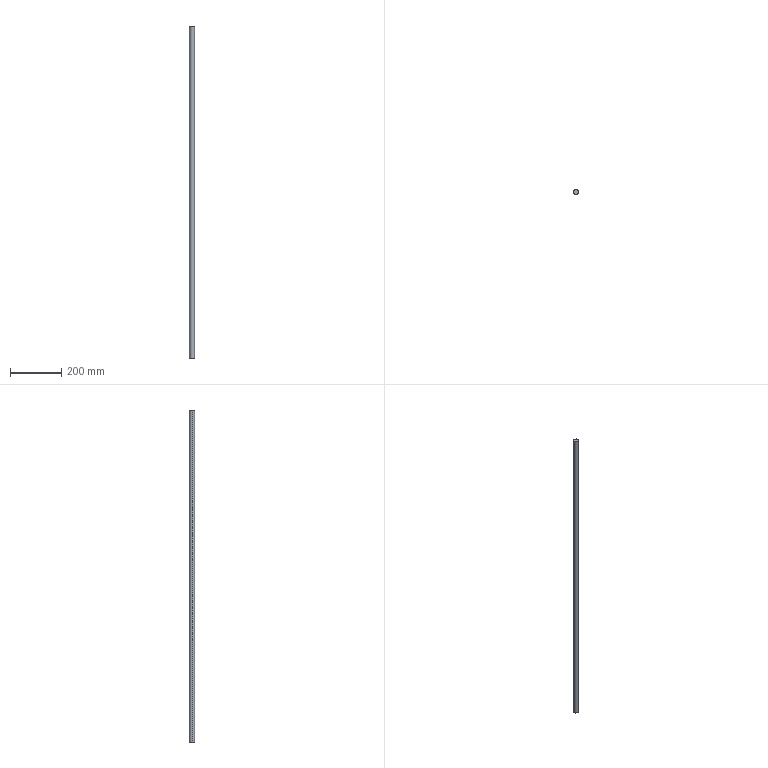Part | SolidWorks | features Extrusion 1 | 1 solid | 4 faces | box 20 x 20 x 1300 mm | volume 408407 mm3 | cylinder 2 | plane 2 | commonest cylinder face diameters 20 x2
STEP:
#1=CARTESIAN_POINT('',(10.,0.,650.));
#2=VERTEX_POINT('',#1);
#3=CARTESIAN_POINT('',(-10.,0.,650.));
#4=VERTEX_POINT('',#3);
#5=CARTESIAN_POINT('',(0.,0.,650.));
#6=DIRECTION('',(0.,0.,1.));
#7=DIRECTION('',(1.,0.,0.));
#8=AXIS2_PLACEMENT_3D('',#5,#6,#7);
#9=CIRCLE('',#8,10.);
#10=EDGE_CURVE('',#2,#4,#9,.T.);
#11=ORIENTED_EDGE('',*,*,#10,.F.);
#12=CARTESIAN_POINT('',(10.,0.,-650.));
#13=VERTEX_POINT('',#12);
#14=CARTESIAN_POINT('',(10.,0.,650.));
#15=DIRECTION('',(0.,0.,-1.));
#16=VECTOR('',#15,1000.);
#17=LINE('',#14,#16);
#18=EDGE_CURVE('',#2,#13,#17,.T.);
#19=ORIENTED_EDGE('',*,*,#18,.T.);
#20=CARTESIAN_POINT('',(-10.,0.,-650.));
#21=VERTEX_POINT('',#20);
#22=CARTESIAN_POINT('',(0.,0.,-650.));
#23=DIRECTION('',(0.,0.,1.));
#24=DIRECTION('',(1.,0.,0.));
#25=AXIS2_PLACEMENT_3D('',#22,#23,#24);
#26=CIRCLE('',#25,10.);
#27=EDGE_CURVE('',#13,#21,#26,.T.);
#28=ORIENTED_EDGE('',*,*,#27,.T.);
#29=CARTESIAN_POINT('',(-10.,0.,650.));
#30=DIRECTION('',(0.,0.,-1.));
#31=VECTOR('',#30,1000.);
#32=LINE('',#29,#31);
#33=EDGE_CURVE('',#4,#21,#32,.T.);
#34=ORIENTED_EDGE('',*,*,#33,.F.);
#35=EDGE_LOOP('',(#11,#19,#28,#34));
#36=FACE_OUTER_BOUND('',#35,.T.);
#37=CARTESIAN_POINT('',(0.,0.,650.));
#38=DIRECTION('',(0.,0.,-1.));
#39=DIRECTION('',(-1.,0.,0.));
#40=AXIS2_PLACEMENT_3D('',#37,#38,#39);
#41=CYLINDRICAL_SURFACE('',#40,10.);
#42=ADVANCED_FACE('',(#36),#41,.T.);
#43=ORIENTED_EDGE('',*,*,#18,.F.);
#44=CARTESIAN_POINT('',(0.,0.,650.));
#45=DIRECTION('',(0.,0.,1.));
#46=DIRECTION('',(1.,0.,0.));
#47=AXIS2_PLACEMENT_3D('',#44,#45,#46);
#48=CIRCLE('',#47,10.);
#49=EDGE_CURVE('',#4,#2,#48,.T.);
#50=ORIENTED_EDGE('',*,*,#49,.F.);
#51=ORIENTED_EDGE('',*,*,#33,.T.);
#52=CARTESIAN_POINT('',(0.,0.,-650.));
#53=DIRECTION('',(0.,0.,1.));
#54=DIRECTION('',(1.,0.,0.));
#55=AXIS2_PLACEMENT_3D('',#52,#53,#54);
#56=CIRCLE('',#55,10.);
#57=EDGE_CURVE('',#21,#13,#56,.T.);
#58=ORIENTED_EDGE('',*,*,#57,.T.);
#59=EDGE_LOOP('',(#43,#50,#51,#58));
#60=FACE_OUTER_BOUND('',#59,.T.);
#61=CARTESIAN_POINT('',(0.,0.,650.));
#62=DIRECTION('',(0.,0.,-1.));
#63=DIRECTION('',(-1.,0.,0.));
#64=AXIS2_PLACEMENT_3D('',#61,#62,#63);
#65=CYLINDRICAL_SURFACE('',#64,10.);
#66=ADVANCED_FACE('',(#60),#65,.T.);
#67=ORIENTED_EDGE('',*,*,#49,.T.);
#68=ORIENTED_EDGE('',*,*,#10,.T.);
#69=EDGE_LOOP('',(#67,#68));
#70=FACE_OUTER_BOUND('',#69,.T.);
#71=CARTESIAN_POINT('',(0.,0.,650.));
#72=DIRECTION('',(0.,0.,1.));
#73=DIRECTION('',(1.,0.,0.));
#74=AXIS2_PLACEMENT_3D('',#71,#72,#73);
#75=PLANE('',#74);
#76=ADVANCED_FACE('',(#70),#75,.T.);
#77=ORIENTED_EDGE('',*,*,#57,.F.);
#78=ORIENTED_EDGE('',*,*,#27,.F.);
#79=EDGE_LOOP('',(#77,#78));
#80=FACE_OUTER_BOUND('',#79,.T.);
#81=CARTESIAN_POINT('',(0.,0.,-650.));
#82=DIRECTION('',(0.,0.,1.));
#83=DIRECTION('',(1.,0.,0.));
#84=AXIS2_PLACEMENT_3D('',#81,#82,#83);
#85=PLANE('',#84);
#86=ADVANCED_FACE('',(#80),#85,.F.);
#87=CLOSED_SHELL('',(#42,#66,#76,#86));
#88=MANIFOLD_SOLID_BREP('',#87);
#89=CARTESIAN_POINT('',(0.,0.,0.));
#90=DIRECTION('',(0.,0.,1.));
#91=DIRECTION('',(1.,0.,0.));
#92=AXIS2_PLACEMENT_3D('',#89,#90,#91);
#93=(LENGTH_UNIT()NAMED_UNIT(*)SI_UNIT(.MILLI.,.METRE.));
#94=UNCERTAINTY_MEASURE_WITH_UNIT(LENGTH_MEASURE(0.00001),#93,'','');
#95=(NAMED_UNIT(*)PLANE_ANGLE_UNIT()SI_UNIT($,.RADIAN.));
#96=(NAMED_UNIT(*)SI_UNIT($,.STERADIAN.)SOLID_ANGLE_UNIT());
#97=(GEOMETRIC_REPRESENTATION_CONTEXT(3)GLOBAL_UNCERTAINTY_ASSIGNED_CONTEXT((#94))GLOBAL_UNIT_ASSIGNED_CONTEXT((#93,#95,#96))REPRESENTATION_CONTEXT('',''));
#98=ADVANCED_BREP_SHAPE_REPRESENTATION('',(#88,#92),#97);